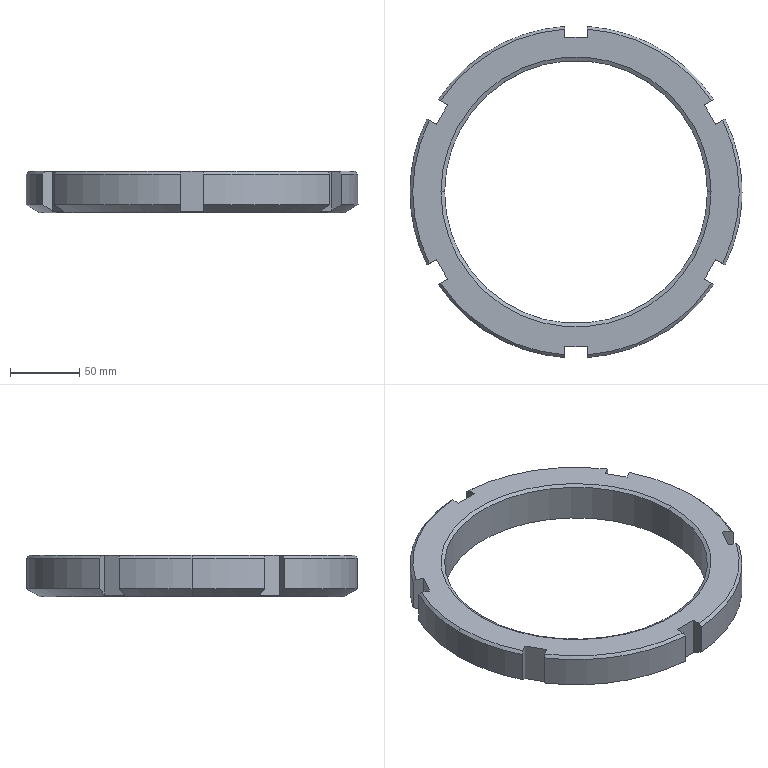Part | SolidWorks | features Chamfer 3, CirPattern 1, Cut 1, Extrusion 1 | 1 solid | 42 faces | box 240 x 239.437 x 30 mm | volume 460595 mm3 | plane 20 | cone 13 | cylinder 9 | commonest cylinder face diameters 240 x7 190 x2
STEP:
#1=CARTESIAN_POINT('',(-95.,0.,28.5));
#2=VERTEX_POINT('',#1);
#3=CARTESIAN_POINT('',(95.,0.,28.5));
#4=VERTEX_POINT('',#3);
#5=CARTESIAN_POINT('',(0.,0.,28.5));
#6=DIRECTION('',(0.,0.,1.));
#7=DIRECTION('',(1.,0.,0.));
#8=AXIS2_PLACEMENT_3D('',#5,#6,#7);
#9=CIRCLE('',#8,95.);
#10=EDGE_CURVE('',#2,#4,#9,.T.);
#11=ORIENTED_EDGE('',*,*,#10,.F.);
#12=CARTESIAN_POINT('',(-97.598,0.,30.));
#13=VERTEX_POINT('',#12);
#14=CARTESIAN_POINT('',(-95.,0.,28.5));
#15=DIRECTION('',(-0.866,0.,0.5));
#16=VECTOR('',#15,1000.);
#17=LINE('',#14,#16);
#18=EDGE_CURVE('',#2,#13,#17,.T.);
#19=ORIENTED_EDGE('',*,*,#18,.T.);
#20=CARTESIAN_POINT('',(97.598,0.,30.));
#21=VERTEX_POINT('',#20);
#22=CARTESIAN_POINT('',(0.,0.,30.));
#23=DIRECTION('',(0.,0.,-1.));
#24=DIRECTION('',(1.,0.,0.));
#25=AXIS2_PLACEMENT_3D('',#22,#23,#24);
#26=CIRCLE('',#25,97.598);
#27=EDGE_CURVE('',#21,#13,#26,.T.);
#28=ORIENTED_EDGE('',*,*,#27,.F.);
#29=CARTESIAN_POINT('',(95.,0.,28.5));
#30=DIRECTION('',(0.866,0.,0.5));
#31=VECTOR('',#30,1000.);
#32=LINE('',#29,#31);
#33=EDGE_CURVE('',#4,#21,#32,.T.);
#34=ORIENTED_EDGE('',*,*,#33,.F.);
#35=EDGE_LOOP('',(#11,#19,#28,#34));
#36=FACE_OUTER_BOUND('',#35,.T.);
#37=CARTESIAN_POINT('',(0.,0.,28.5));
#38=DIRECTION('',(0.,0.,1.));
#39=DIRECTION('',(1.,0.,0.));
#40=AXIS2_PLACEMENT_3D('',#37,#38,#39);
#41=CONICAL_SURFACE('',#40,95.,1.047);
#42=ADVANCED_FACE('',(#36),#41,.F.);
#43=CARTESIAN_POINT('',(95.,0.,1.5));
#44=VERTEX_POINT('',#43);
#45=CARTESIAN_POINT('',(-95.,0.,1.5));
#46=VERTEX_POINT('',#45);
#47=CARTESIAN_POINT('',(0.,0.,1.5));
#48=DIRECTION('',(0.,0.,-1.));
#49=DIRECTION('',(1.,0.,0.));
#50=AXIS2_PLACEMENT_3D('',#47,#48,#49);
#51=CIRCLE('',#50,95.);
#52=EDGE_CURVE('',#44,#46,#51,.T.);
#53=ORIENTED_EDGE('',*,*,#52,.F.);
#54=CARTESIAN_POINT('',(97.598,0.,0.));
#55=VERTEX_POINT('',#54);
#56=CARTESIAN_POINT('',(97.598,0.,0.));
#57=DIRECTION('',(0.866,0.,-0.5));
#58=VECTOR('',#57,1000.);
#59=LINE('',#56,#58);
#60=EDGE_CURVE('',#44,#55,#59,.T.);
#61=ORIENTED_EDGE('',*,*,#60,.T.);
#62=CARTESIAN_POINT('',(-97.598,0.,0.));
#63=VERTEX_POINT('',#62);
#64=CARTESIAN_POINT('',(0.,0.,0.));
#65=DIRECTION('',(0.,0.,1.));
#66=DIRECTION('',(1.,0.,0.));
#67=AXIS2_PLACEMENT_3D('',#64,#65,#66);
#68=CIRCLE('',#67,97.598);
#69=EDGE_CURVE('',#63,#55,#68,.T.);
#70=ORIENTED_EDGE('',*,*,#69,.F.);
#71=CARTESIAN_POINT('',(-97.598,0.,0.));
#72=DIRECTION('',(-0.866,0.,-0.5));
#73=VECTOR('',#72,1000.);
#74=LINE('',#71,#73);
#75=EDGE_CURVE('',#46,#63,#74,.T.);
#76=ORIENTED_EDGE('',*,*,#75,.F.);
#77=EDGE_LOOP('',(#53,#61,#70,#76));
#78=FACE_OUTER_BOUND('',#77,.T.);
#79=CARTESIAN_POINT('',(0.,0.,0.));
#80=DIRECTION('',(0.,0.,-1.));
#81=DIRECTION('',(-1.,0.,0.));
#82=AXIS2_PLACEMENT_3D('',#79,#80,#81);
#83=CONICAL_SURFACE('',#82,97.598,1.047);
#84=ADVANCED_FACE('',(#78),#83,.F.);
#85=CARTESIAN_POINT('',(-110.,0.,0.));
#86=VERTEX_POINT('',#85);
#87=CARTESIAN_POINT('',(110.,0.,0.));
#88=VERTEX_POINT('',#87);
#89=CARTESIAN_POINT('',(0.,0.,0.));
#90=DIRECTION('',(0.,0.,-1.));
#91=DIRECTION('',(1.,0.,0.));
#92=AXIS2_PLACEMENT_3D('',#89,#90,#91);
#93=CIRCLE('',#92,110.);
#94=EDGE_CURVE('',#86,#88,#93,.T.);
#95=ORIENTED_EDGE('',*,*,#94,.F.);
#96=CARTESIAN_POINT('',(-120.,0.,5.774));
#97=VERTEX_POINT('',#96);
#98=CARTESIAN_POINT('',(-120.,0.,5.774));
#99=DIRECTION('',(-0.866,0.,0.5));
#100=VECTOR('',#99,1000.);
#101=LINE('',#98,#100);
#102=EDGE_CURVE('',#86,#97,#101,.T.);
#103=ORIENTED_EDGE('',*,*,#102,.T.);
#104=CARTESIAN_POINT('',(-107.787,52.745,5.774));
#105=VERTEX_POINT('',#104);
#106=CARTESIAN_POINT('',(0.,0.,5.774));
#107=DIRECTION('',(0.,0.,1.));
#108=DIRECTION('',(1.,0.,0.));
#109=AXIS2_PLACEMENT_3D('',#106,#107,#108);
#110=CIRCLE('',#109,120.);
#111=EDGE_CURVE('',#105,#97,#110,.T.);
#112=ORIENTED_EDGE('',*,*,#111,.F.);
#113=CARTESIAN_POINT('',(-100.945,48.795,1.224));
#114=VERTEX_POINT('',#113);
#115=CARTESIAN_POINT('',(-100.945,48.795,1.224));
#116=CARTESIAN_POINT('',(-103.226,50.112,2.74));
#117=CARTESIAN_POINT('',(-105.506,51.428,4.257));
#118=CARTESIAN_POINT('',(-107.787,52.745,5.774));
#119=B_SPLINE_CURVE_WITH_KNOTS('',3,(#115,#116,#117,#118),.UNSPECIFIED.,.F.,.F.,(4,4),(0.000000267,0.009117),.UNSPECIFIED.);
#120=EDGE_CURVE('',#114,#105,#119,.T.);
#121=ORIENTED_EDGE('',*,*,#120,.F.);
#122=CARTESIAN_POINT('',(-92.73,63.024,1.224));
#123=VERTEX_POINT('',#122);
#124=CARTESIAN_POINT('',(-92.73,63.024,1.224));
#125=CARTESIAN_POINT('',(-95.468,58.281,0.9922));
#126=CARTESIAN_POINT('',(-98.207,53.538,0.9922));
#127=CARTESIAN_POINT('',(-100.945,48.795,1.224));
#128=B_SPLINE_CURVE_WITH_KNOTS('',3,(#124,#125,#126,#127),.UNSPECIFIED.,.F.,.F.,(4,4),(0.000000231,0.01643),.UNSPECIFIED.);
#129=EDGE_CURVE('',#123,#114,#128,.T.);
#130=ORIENTED_EDGE('',*,*,#129,.F.);
#131=CARTESIAN_POINT('',(-99.572,66.974,5.774));
#132=VERTEX_POINT('',#131);
#133=CARTESIAN_POINT('',(-99.572,66.974,5.774));
#134=CARTESIAN_POINT('',(-97.291,65.657,4.257));
#135=CARTESIAN_POINT('',(-95.011,64.34,2.74));
#136=CARTESIAN_POINT('',(-92.73,63.024,1.224));
#137=B_SPLINE_CURVE_WITH_KNOTS('',3,(#133,#134,#135,#136),.UNSPECIFIED.,.F.,.F.,(4,4),(0.000000267,0.009117),.UNSPECIFIED.);
#138=EDGE_CURVE('',#132,#123,#137,.T.);
#139=ORIENTED_EDGE('',*,*,#138,.F.);
#140=CARTESIAN_POINT('',(-8.215,119.718,5.774));
#141=VERTEX_POINT('',#140);
#142=CARTESIAN_POINT('',(0.,0.,5.774));
#143=DIRECTION('',(0.,0.,1.));
#144=DIRECTION('',(1.,0.,0.));
#145=AXIS2_PLACEMENT_3D('',#142,#143,#144);
#146=CIRCLE('',#145,120.);
#147=EDGE_CURVE('',#141,#132,#146,.T.);
#148=ORIENTED_EDGE('',*,*,#147,.F.);
#149=CARTESIAN_POINT('',(-8.215,111.818,1.224));
#150=VERTEX_POINT('',#149);
#151=CARTESIAN_POINT('',(-8.215,111.818,1.224));
#152=CARTESIAN_POINT('',(-8.215,112.097,1.384));
#153=CARTESIAN_POINT('',(-8.215,112.376,1.545));
#154=CARTESIAN_POINT('',(-8.215,112.655,1.706));
#155=CARTESIAN_POINT('',(-8.215,115.01,3.061));
#156=CARTESIAN_POINT('',(-8.215,117.364,4.417));
#157=CARTESIAN_POINT('',(-8.215,119.718,5.774));
#158=B_SPLINE_CURVE_WITH_KNOTS('',3,(#151,#152,#153,#154,#155,#156,#157),.UNSPECIFIED.,.F.,.F.,(4,3,4),(0.0177,0.01867,0.02682),.UNSPECIFIED.);
#159=EDGE_CURVE('',#150,#141,#158,.T.);
#160=ORIENTED_EDGE('',*,*,#159,.F.);
#161=CARTESIAN_POINT('',(8.215,111.818,1.224));
#162=VERTEX_POINT('',#161);
#163=CARTESIAN_POINT('',(8.215,111.818,1.224));
#164=CARTESIAN_POINT('',(5.483,111.818,1.108));
#165=CARTESIAN_POINT('',(2.747,111.818,1.05));
#166=CARTESIAN_POINT('',(-2.73,111.818,1.05));
#167=CARTESIAN_POINT('',(-5.475,111.818,1.108));
#168=CARTESIAN_POINT('',(-8.215,111.818,1.224));
#169=B_SPLINE_CURVE_WITH_KNOTS('',3,(#163,#164,#165,#166,#167,#168),.UNSPECIFIED.,.F.,.F.,(4,2,4),(0.01999,0.02819,0.0364),.UNSPECIFIED.);
#170=EDGE_CURVE('',#162,#150,#169,.T.);
#171=ORIENTED_EDGE('',*,*,#170,.F.);
#172=CARTESIAN_POINT('',(8.215,119.718,5.774));
#173=VERTEX_POINT('',#172);
#174=CARTESIAN_POINT('',(8.215,119.718,5.774));
#175=CARTESIAN_POINT('',(8.215,117.364,4.417));
#176=CARTESIAN_POINT('',(8.215,115.01,3.061));
#177=CARTESIAN_POINT('',(8.215,112.655,1.706));
#178=CARTESIAN_POINT('',(8.215,112.376,1.545));
#179=CARTESIAN_POINT('',(8.215,112.097,1.384));
#180=CARTESIAN_POINT('',(8.215,111.818,1.224));
#181=B_SPLINE_CURVE_WITH_KNOTS('',3,(#174,#175,#176,#177,#178,#179,#180),.UNSPECIFIED.,.F.,.F.,(4,3,4),(0.01052,0.01867,0.01963),.UNSPECIFIED.);
#182=EDGE_CURVE('',#173,#162,#181,.T.);
#183=ORIENTED_EDGE('',*,*,#182,.F.);
#184=CARTESIAN_POINT('',(99.572,66.974,5.774));
#185=VERTEX_POINT('',#184);
#186=CARTESIAN_POINT('',(0.,0.,5.774));
#187=DIRECTION('',(0.,0.,1.));
#188=DIRECTION('',(1.,0.,0.));
#189=AXIS2_PLACEMENT_3D('',#186,#187,#188);
#190=CIRCLE('',#189,120.);
#191=EDGE_CURVE('',#185,#173,#190,.T.);
#192=ORIENTED_EDGE('',*,*,#191,.F.);
#193=CARTESIAN_POINT('',(92.73,63.024,1.224));
#194=VERTEX_POINT('',#193);
#195=CARTESIAN_POINT('',(92.73,63.024,1.224));
#196=CARTESIAN_POINT('',(95.011,64.34,2.74));
#197=CARTESIAN_POINT('',(97.291,65.657,4.257));
#198=CARTESIAN_POINT('',(99.572,66.974,5.774));
#199=B_SPLINE_CURVE_WITH_KNOTS('',3,(#195,#196,#197,#198),.UNSPECIFIED.,.F.,.F.,(4,4),(0.000000267,0.009117),.UNSPECIFIED.);
#200=EDGE_CURVE('',#194,#185,#199,.T.);
#201=ORIENTED_EDGE('',*,*,#200,.F.);
#202=CARTESIAN_POINT('',(100.945,48.795,1.224));
#203=VERTEX_POINT('',#202);
#204=CARTESIAN_POINT('',(100.945,48.795,1.224));
#205=CARTESIAN_POINT('',(98.207,53.538,0.9922));
#206=CARTESIAN_POINT('',(95.468,58.281,0.9922));
#207=CARTESIAN_POINT('',(92.73,63.024,1.224));
#208=B_SPLINE_CURVE_WITH_KNOTS('',3,(#204,#205,#206,#207),.UNSPECIFIED.,.F.,.F.,(4,4),(0.000000231,0.01643),.UNSPECIFIED.);
#209=EDGE_CURVE('',#203,#194,#208,.T.);
#210=ORIENTED_EDGE('',*,*,#209,.F.);
#211=CARTESIAN_POINT('',(107.787,52.745,5.774));
#212=VERTEX_POINT('',#211);
#213=CARTESIAN_POINT('',(107.787,52.745,5.774));
#214=CARTESIAN_POINT('',(105.506,51.428,4.257));
#215=CARTESIAN_POINT('',(103.226,50.112,2.74));
#216=CARTESIAN_POINT('',(100.945,48.795,1.224));
#217=B_SPLINE_CURVE_WITH_KNOTS('',3,(#213,#214,#215,#216),.UNSPECIFIED.,.F.,.F.,(4,4),(0.000000267,0.009117),.UNSPECIFIED.);
#218=EDGE_CURVE('',#212,#203,#217,.T.);
#219=ORIENTED_EDGE('',*,*,#218,.F.);
#220=CARTESIAN_POINT('',(120.,0.,5.774));
#221=VERTEX_POINT('',#220);
#222=CARTESIAN_POINT('',(0.,0.,5.774));
#223=DIRECTION('',(0.,0.,1.));
#224=DIRECTION('',(1.,0.,0.));
#225=AXIS2_PLACEMENT_3D('',#222,#223,#224);
#226=CIRCLE('',#225,120.);
#227=EDGE_CURVE('',#221,#212,#226,.T.);
#228=ORIENTED_EDGE('',*,*,#227,.F.);
#229=CARTESIAN_POINT('',(120.,0.,5.774));
#230=DIRECTION('',(0.866,0.,0.5));
#231=VECTOR('',#230,1000.);
#232=LINE('',#229,#231);
#233=EDGE_CURVE('',#88,#221,#232,.T.);
#234=ORIENTED_EDGE('',*,*,#233,.F.);
#235=EDGE_LOOP('',(#95,#103,#112,#121,#130,#139,#148,#160,#171,#183,#192,#201,#210,#219,#228,#234));
#236=FACE_OUTER_BOUND('',#235,.T.);
#237=CARTESIAN_POINT('',(0.,0.,5.774));
#238=DIRECTION('',(0.,0.,1.));
#239=DIRECTION('',(1.,0.,0.));
#240=AXIS2_PLACEMENT_3D('',#237,#238,#239);
#241=CONICAL_SURFACE('',#240,120.,1.047);
#242=ADVANCED_FACE('',(#236),#241,.T.);
#243=ORIENTED_EDGE('',*,*,#10,.T.);
#244=CARTESIAN_POINT('',(95.,0.,30.));
#245=DIRECTION('',(0.,0.,-1.));
#246=VECTOR('',#245,1000.);
#247=LINE('',#244,#246);
#248=EDGE_CURVE('',#4,#44,#247,.T.);
#249=ORIENTED_EDGE('',*,*,#248,.T.);
#250=ORIENTED_EDGE('',*,*,#52,.T.);
#251=CARTESIAN_POINT('',(-95.,0.,30.));
#252=DIRECTION('',(0.,0.,-1.));
#253=VECTOR('',#252,1000.);
#254=LINE('',#251,#253);
#255=EDGE_CURVE('',#2,#46,#254,.T.);
#256=ORIENTED_EDGE('',*,*,#255,.F.);
#257=EDGE_LOOP('',(#243,#249,#250,#256));
#258=FACE_OUTER_BOUND('',#257,.T.);
#259=CARTESIAN_POINT('',(0.,0.,30.));
#260=DIRECTION('',(0.,0.,-1.));
#261=DIRECTION('',(-1.,0.,0.));
#262=AXIS2_PLACEMENT_3D('',#259,#260,#261);
#263=CYLINDRICAL_SURFACE('',#262,95.);
#264=ADVANCED_FACE('',(#258),#263,.F.);
#265=CARTESIAN_POINT('',(-118.,0.,30.));
#266=VERTEX_POINT('',#265);
#267=CARTESIAN_POINT('',(-106.051,-51.742,30.));
#268=VERTEX_POINT('',#267);
#269=CARTESIAN_POINT('',(0.,0.,30.));
#270=DIRECTION('',(0.,0.,1.));
#271=DIRECTION('',(1.,0.,0.));
#272=AXIS2_PLACEMENT_3D('',#269,#270,#271);
#273=CIRCLE('',#272,118.);
#274=EDGE_CURVE('',#266,#268,#273,.T.);
#275=ORIENTED_EDGE('',*,*,#274,.F.);
#276=CARTESIAN_POINT('',(-120.,0.,28.));
#277=VERTEX_POINT('',#276);
#278=CARTESIAN_POINT('',(-118.,0.,30.));
#279=DIRECTION('',(-0.7071,0.,-0.7071));
#280=VECTOR('',#279,1000.);
#281=LINE('',#278,#280);
#282=EDGE_CURVE('',#266,#277,#281,.T.);
#283=ORIENTED_EDGE('',*,*,#282,.T.);
#284=CARTESIAN_POINT('',(-107.787,-52.745,28.));
#285=VERTEX_POINT('',#284);
#286=CARTESIAN_POINT('',(0.,0.,28.));
#287=DIRECTION('',(0.,0.,-1.));
#288=DIRECTION('',(1.,0.,0.));
#289=AXIS2_PLACEMENT_3D('',#286,#287,#288);
#290=CIRCLE('',#289,120.);
#291=EDGE_CURVE('',#285,#277,#290,.T.);
#292=ORIENTED_EDGE('',*,*,#291,.F.);
#293=CARTESIAN_POINT('',(-106.051,-51.742,30.));
#294=CARTESIAN_POINT('',(-106.629,-52.077,29.333));
#295=CARTESIAN_POINT('',(-107.208,-52.411,28.667));
#296=CARTESIAN_POINT('',(-107.787,-52.745,28.));
#297=B_SPLINE_CURVE_WITH_KNOTS('',3,(#293,#294,#295,#296),.UNSPECIFIED.,.F.,.F.,(4,4),(0.000000283,0.002832),.UNSPECIFIED.);
#298=EDGE_CURVE('',#268,#285,#297,.T.);
#299=ORIENTED_EDGE('',*,*,#298,.F.);
#300=EDGE_LOOP('',(#275,#283,#292,#299));
#301=FACE_OUTER_BOUND('',#300,.T.);
#302=CARTESIAN_POINT('',(0.,0.,30.));
#303=DIRECTION('',(0.,0.,-1.));
#304=DIRECTION('',(-1.,0.,0.));
#305=AXIS2_PLACEMENT_3D('',#302,#303,#304);
#306=CONICAL_SURFACE('',#305,118.,0.7854);
#307=ADVANCED_FACE('',(#301),#306,.T.);
#308=ORIENTED_EDGE('',*,*,#291,.T.);
#309=CARTESIAN_POINT('',(-120.,0.,30.));
#310=DIRECTION('',(0.,0.,-1.));
#311=VECTOR('',#310,1000.);
#312=LINE('',#309,#311);
#313=EDGE_CURVE('',#277,#97,#312,.T.);
#314=ORIENTED_EDGE('',*,*,#313,.T.);
#315=CARTESIAN_POINT('',(-107.787,-52.745,5.774));
#316=VERTEX_POINT('',#315);
#317=CARTESIAN_POINT('',(0.,0.,5.774));
#318=DIRECTION('',(0.,0.,1.));
#319=DIRECTION('',(1.,0.,0.));
#320=AXIS2_PLACEMENT_3D('',#317,#318,#319);
#321=CIRCLE('',#320,120.);
#322=EDGE_CURVE('',#97,#316,#321,.T.);
#323=ORIENTED_EDGE('',*,*,#322,.T.);
#324=CARTESIAN_POINT('',(-107.787,-52.745,0.));
#325=DIRECTION('',(0.,0.,1.));
#326=VECTOR('',#325,1000.);
#327=LINE('',#324,#326);
#328=EDGE_CURVE('',#316,#285,#327,.T.);
#329=ORIENTED_EDGE('',*,*,#328,.T.);
#330=EDGE_LOOP('',(#308,#314,#323,#329));
#331=FACE_OUTER_BOUND('',#330,.T.);
#332=CARTESIAN_POINT('',(0.,0.,30.));
#333=DIRECTION('',(0.,0.,-1.));
#334=DIRECTION('',(-1.,0.,0.));
#335=AXIS2_PLACEMENT_3D('',#332,#333,#334);
#336=CYLINDRICAL_SURFACE('',#335,120.);
#337=ADVANCED_FACE('',(#331),#336,.T.);
#338=CARTESIAN_POINT('',(107.787,52.745,28.));
#339=VERTEX_POINT('',#338);
#340=CARTESIAN_POINT('',(107.787,-52.745,28.));
#341=VERTEX_POINT('',#340);
#342=CARTESIAN_POINT('',(0.,0.,28.));
#343=DIRECTION('',(0.,0.,-1.));
#344=DIRECTION('',(1.,0.,0.));
#345=AXIS2_PLACEMENT_3D('',#342,#343,#344);
#346=CIRCLE('',#345,120.);
#347=EDGE_CURVE('',#339,#341,#346,.T.);
#348=ORIENTED_EDGE('',*,*,#347,.T.);
#349=CARTESIAN_POINT('',(107.787,-52.745,5.774));
#350=VERTEX_POINT('',#349);
#351=CARTESIAN_POINT('',(107.787,-52.745,0.));
#352=DIRECTION('',(0.,0.,1.));
#353=VECTOR('',#352,1000.);
#354=LINE('',#351,#353);
#355=EDGE_CURVE('',#350,#341,#354,.T.);
#356=ORIENTED_EDGE('',*,*,#355,.F.);
#357=CARTESIAN_POINT('',(0.,0.,5.774));
#358=DIRECTION('',(0.,0.,1.));
#359=DIRECTION('',(1.,0.,0.));
#360=AXIS2_PLACEMENT_3D('',#357,#358,#359);
#361=CIRCLE('',#360,120.);
#362=EDGE_CURVE('',#350,#221,#361,.T.);
#363=ORIENTED_EDGE('',*,*,#362,.T.);
#364=ORIENTED_EDGE('',*,*,#227,.T.);
#365=CARTESIAN_POINT('',(107.787,52.745,0.));
#366=DIRECTION('',(0.,0.,1.));
#367=VECTOR('',#366,1000.);
#368=LINE('',#365,#367);
#369=EDGE_CURVE('',#212,#339,#368,.T.);
#370=ORIENTED_EDGE('',*,*,#369,.T.);
#371=EDGE_LOOP('',(#348,#356,#363,#364,#370));
#372=FACE_OUTER_BOUND('',#371,.T.);
#373=CARTESIAN_POINT('',(0.,0.,30.));
#374=DIRECTION('',(0.,0.,-1.));
#375=DIRECTION('',(-1.,0.,0.));
#376=AXIS2_PLACEMENT_3D('',#373,#374,#375);
#377=CYLINDRICAL_SURFACE('',#376,120.);
#378=ADVANCED_FACE('',(#372),#377,.T.);
#379=CARTESIAN_POINT('',(106.051,-51.742,30.));
#380=VERTEX_POINT('',#379);
#381=CARTESIAN_POINT('',(107.787,-52.745,28.));
#382=CARTESIAN_POINT('',(107.208,-52.411,28.667));
#383=CARTESIAN_POINT('',(106.629,-52.077,29.333));
#384=CARTESIAN_POINT('',(106.051,-51.742,30.));
#385=B_SPLINE_CURVE_WITH_KNOTS('',3,(#381,#382,#383,#384),.UNSPECIFIED.,.F.,.F.,(4,4),(0.000000283,0.002832),.UNSPECIFIED.);
#386=EDGE_CURVE('',#341,#380,#385,.T.);
#387=ORIENTED_EDGE('',*,*,#386,.F.);
#388=ORIENTED_EDGE('',*,*,#347,.F.);
#389=CARTESIAN_POINT('',(106.051,51.742,30.));
#390=VERTEX_POINT('',#389);
#391=CARTESIAN_POINT('',(106.051,51.742,30.));
#392=CARTESIAN_POINT('',(106.629,52.077,29.333));
#393=CARTESIAN_POINT('',(107.208,52.411,28.667));
#394=CARTESIAN_POINT('',(107.787,52.745,28.));
#395=B_SPLINE_CURVE_WITH_KNOTS('',3,(#391,#392,#393,#394),.UNSPECIFIED.,.F.,.F.,(4,4),(0.000000283,0.002832),.UNSPECIFIED.);
#396=EDGE_CURVE('',#390,#339,#395,.T.);
#397=ORIENTED_EDGE('',*,*,#396,.F.);
#398=CARTESIAN_POINT('',(0.,0.,30.));
#399=DIRECTION('',(0.,0.,1.));
#400=DIRECTION('',(1.,0.,0.));
#401=AXIS2_PLACEMENT_3D('',#398,#399,#400);
#402=CIRCLE('',#401,118.);
#403=EDGE_CURVE('',#380,#390,#402,.T.);
#404=ORIENTED_EDGE('',*,*,#403,.F.);
#405=EDGE_LOOP('',(#387,#388,#397,#404));
#406=FACE_OUTER_BOUND('',#405,.T.);
#407=CARTESIAN_POINT('',(0.,0.,30.));
#408=DIRECTION('',(0.,0.,-1.));
#409=DIRECTION('',(-1.,0.,0.));
#410=AXIS2_PLACEMENT_3D('',#407,#408,#409);
#411=CONICAL_SURFACE('',#410,118.,0.7854);
#412=ADVANCED_FACE('',(#406),#411,.T.);
#413=CARTESIAN_POINT('',(8.215,119.718,28.));
#414=VERTEX_POINT('',#413);
#415=CARTESIAN_POINT('',(99.572,66.974,28.));
#416=VERTEX_POINT('',#415);
#417=CARTESIAN_POINT('',(0.,0.,28.));
#418=DIRECTION('',(0.,0.,-1.));
#419=DIRECTION('',(1.,0.,0.));
#420=AXIS2_PLACEMENT_3D('',#417,#418,#419);
#421=CIRCLE('',#420,120.);
#422=EDGE_CURVE('',#414,#416,#421,.T.);
#423=ORIENTED_EDGE('',*,*,#422,.T.);
#424=CARTESIAN_POINT('',(99.572,66.974,0.));
#425=DIRECTION('',(0.,0.,1.));
#426=VECTOR('',#425,1000.);
#427=LINE('',#424,#426);
#428=EDGE_CURVE('',#185,#416,#427,.T.);
#429=ORIENTED_EDGE('',*,*,#428,.F.);
#430=ORIENTED_EDGE('',*,*,#191,.T.);
#431=CARTESIAN_POINT('',(8.215,119.718,0.));
#432=DIRECTION('',(0.,0.,1.));
#433=VECTOR('',#432,1000.);
#434=LINE('',#431,#433);
#435=EDGE_CURVE('',#173,#414,#434,.T.);
#436=ORIENTED_EDGE('',*,*,#435,.T.);
#437=EDGE_LOOP('',(#423,#429,#430,#436));
#438=FACE_OUTER_BOUND('',#437,.T.);
#439=CARTESIAN_POINT('',(0.,0.,30.));
#440=DIRECTION('',(0.,0.,-1.));
#441=DIRECTION('',(-1.,0.,0.));
#442=AXIS2_PLACEMENT_3D('',#439,#440,#441);
#443=CYLINDRICAL_SURFACE('',#442,120.);
#444=ADVANCED_FACE('',(#438),#443,.T.);
#445=CARTESIAN_POINT('',(97.836,65.971,30.));
#446=VERTEX_POINT('',#445);
#447=CARTESIAN_POINT('',(99.572,66.974,28.));
#448=CARTESIAN_POINT('',(98.993,66.64,28.667));
#449=CARTESIAN_POINT('',(98.414,66.305,29.333));
#450=CARTESIAN_POINT('',(97.836,65.971,30.));
#451=B_SPLINE_CURVE_WITH_KNOTS('',3,(#447,#448,#449,#450),.UNSPECIFIED.,.F.,.F.,(4,4),(0.000000283,0.002832),.UNSPECIFIED.);
#452=EDGE_CURVE('',#416,#446,#451,.T.);
#453=ORIENTED_EDGE('',*,*,#452,.F.);
#454=ORIENTED_EDGE('',*,*,#422,.F.);
#455=CARTESIAN_POINT('',(8.215,117.714,30.));
#456=VERTEX_POINT('',#455);
#457=CARTESIAN_POINT('',(8.215,117.714,30.));
#458=CARTESIAN_POINT('',(8.215,117.72,29.993));
#459=CARTESIAN_POINT('',(8.215,117.727,29.987));
#460=CARTESIAN_POINT('',(8.215,117.734,29.98));
#461=CARTESIAN_POINT('',(8.215,118.395,29.32));
#462=CARTESIAN_POINT('',(8.215,119.057,28.66));
#463=CARTESIAN_POINT('',(8.215,119.718,28.));
#464=B_SPLINE_CURVE_WITH_KNOTS('',3,(#457,#458,#459,#460,#461,#462,#463),.UNSPECIFIED.,.F.,.F.,(4,3,4),(0.01541,0.01543,0.01824),.UNSPECIFIED.);
#465=EDGE_CURVE('',#456,#414,#464,.T.);
#466=ORIENTED_EDGE('',*,*,#465,.F.);
#467=CARTESIAN_POINT('',(0.,0.,30.));
#468=DIRECTION('',(0.,0.,1.));
#469=DIRECTION('',(1.,0.,0.));
#470=AXIS2_PLACEMENT_3D('',#467,#468,#469);
#471=CIRCLE('',#470,118.);
#472=EDGE_CURVE('',#446,#456,#471,.T.);
#473=ORIENTED_EDGE('',*,*,#472,.F.);
#474=EDGE_LOOP('',(#453,#454,#466,#473));
#475=FACE_OUTER_BOUND('',#474,.T.);
#476=CARTESIAN_POINT('',(0.,0.,30.));
#477=DIRECTION('',(0.,0.,-1.));
#478=DIRECTION('',(-1.,0.,0.));
#479=AXIS2_PLACEMENT_3D('',#476,#477,#478);
#480=CONICAL_SURFACE('',#479,118.,0.7854);
#481=ADVANCED_FACE('',(#475),#480,.T.);
#482=CARTESIAN_POINT('',(-99.572,66.974,28.));
#483=VERTEX_POINT('',#482);
#484=CARTESIAN_POINT('',(-8.215,119.718,28.));
#485=VERTEX_POINT('',#484);
#486=CARTESIAN_POINT('',(0.,0.,28.));
#487=DIRECTION('',(0.,0.,-1.));
#488=DIRECTION('',(1.,0.,0.));
#489=AXIS2_PLACEMENT_3D('',#486,#487,#488);
#490=CIRCLE('',#489,120.);
#491=EDGE_CURVE('',#483,#485,#490,.T.);
#492=ORIENTED_EDGE('',*,*,#491,.T.);
#493=CARTESIAN_POINT('',(-8.215,119.718,0.));
#494=DIRECTION('',(0.,0.,1.));
#495=VECTOR('',#494,1000.);
#496=LINE('',#493,#495);
#497=EDGE_CURVE('',#141,#485,#496,.T.);
#498=ORIENTED_EDGE('',*,*,#497,.F.);
#499=ORIENTED_EDGE('',*,*,#147,.T.);
#500=CARTESIAN_POINT('',(-99.572,66.974,0.));
#501=DIRECTION('',(0.,0.,1.));
#502=VECTOR('',#501,1000.);
#503=LINE('',#500,#502);
#504=EDGE_CURVE('',#132,#483,#503,.T.);
#505=ORIENTED_EDGE('',*,*,#504,.T.);
#506=EDGE_LOOP('',(#492,#498,#499,#505));
#507=FACE_OUTER_BOUND('',#506,.T.);
#508=CARTESIAN_POINT('',(0.,0.,30.));
#509=DIRECTION('',(0.,0.,-1.));
#510=DIRECTION('',(-1.,0.,0.));
#511=AXIS2_PLACEMENT_3D('',#508,#509,#510);
#512=CYLINDRICAL_SURFACE('',#511,120.);
#513=ADVANCED_FACE('',(#507),#512,.T.);
#514=CARTESIAN_POINT('',(-8.215,117.714,30.));
#515=VERTEX_POINT('',#514);
#516=CARTESIAN_POINT('',(-8.215,119.718,28.));
#517=CARTESIAN_POINT('',(-8.215,119.057,28.66));
#518=CARTESIAN_POINT('',(-8.215,118.395,29.32));
#519=CARTESIAN_POINT('',(-8.215,117.734,29.98));
#520=CARTESIAN_POINT('',(-8.215,117.727,29.987));
#521=CARTESIAN_POINT('',(-8.215,117.72,29.993));
#522=CARTESIAN_POINT('',(-8.215,117.714,30.));
#523=B_SPLINE_CURVE_WITH_KNOTS('',3,(#516,#517,#518,#519,#520,#521,#522),.UNSPECIFIED.,.F.,.F.,(4,3,4),(0.01263,0.01543,0.01546),.UNSPECIFIED.);
#524=EDGE_CURVE('',#485,#515,#523,.T.);
#525=ORIENTED_EDGE('',*,*,#524,.F.);
#526=ORIENTED_EDGE('',*,*,#491,.F.);
#527=CARTESIAN_POINT('',(-97.836,65.971,30.));
#528=VERTEX_POINT('',#527);
#529=CARTESIAN_POINT('',(-97.836,65.971,30.));
#530=CARTESIAN_POINT('',(-98.414,66.305,29.333));
#531=CARTESIAN_POINT('',(-98.993,66.64,28.667));
#532=CARTESIAN_POINT('',(-99.572,66.974,28.));
#533=B_SPLINE_CURVE_WITH_KNOTS('',3,(#529,#530,#531,#532),.UNSPECIFIED.,.F.,.F.,(4,4),(0.000000283,0.002832),.UNSPECIFIED.);
#534=EDGE_CURVE('',#528,#483,#533,.T.);
#535=ORIENTED_EDGE('',*,*,#534,.F.);
#536=CARTESIAN_POINT('',(0.,0.,30.));
#537=DIRECTION('',(0.,0.,1.));
#538=DIRECTION('',(1.,0.,0.));
#539=AXIS2_PLACEMENT_3D('',#536,#537,#538);
#540=CIRCLE('',#539,118.);
#541=EDGE_CURVE('',#515,#528,#540,.T.);
#542=ORIENTED_EDGE('',*,*,#541,.F.);
#543=EDGE_LOOP('',(#525,#526,#535,#542));
#544=FACE_OUTER_BOUND('',#543,.T.);
#545=CARTESIAN_POINT('',(0.,0.,30.));
#546=DIRECTION('',(0.,0.,-1.));
#547=DIRECTION('',(-1.,0.,0.));
#548=AXIS2_PLACEMENT_3D('',#545,#546,#547);
#549=CONICAL_SURFACE('',#548,118.,0.7854);
#550=ADVANCED_FACE('',(#544),#549,.T.);
#551=ORIENTED_EDGE('',*,*,#313,.F.);
#552=CARTESIAN_POINT('',(-107.787,52.745,28.));
#553=VERTEX_POINT('',#552);
#554=CARTESIAN_POINT('',(0.,0.,28.));
#555=DIRECTION('',(0.,0.,-1.));
#556=DIRECTION('',(1.,0.,0.));
#557=AXIS2_PLACEMENT_3D('',#554,#555,#556);
#558=CIRCLE('',#557,120.);
#559=EDGE_CURVE('',#277,#553,#558,.T.);
#560=ORIENTED_EDGE('',*,*,#559,.T.);
#561=CARTESIAN_POINT('',(-107.787,52.745,0.));
#562=DIRECTION('',(0.,0.,1.));
#563=VECTOR('',#562,1000.);
#564=LINE('',#561,#563);
#565=EDGE_CURVE('',#105,#553,#564,.T.);
#566=ORIENTED_EDGE('',*,*,#565,.F.);
#567=ORIENTED_EDGE('',*,*,#111,.T.);
#568=EDGE_LOOP('',(#551,#560,#566,#567));
#569=FACE_OUTER_BOUND('',#568,.T.);
#570=CARTESIAN_POINT('',(0.,0.,30.));
#571=DIRECTION('',(0.,0.,-1.));
#572=DIRECTION('',(-1.,0.,0.));
#573=AXIS2_PLACEMENT_3D('',#570,#571,#572);
#574=CYLINDRICAL_SURFACE('',#573,120.);
#575=ADVANCED_FACE('',(#569),#574,.T.);
#576=ORIENTED_EDGE('',*,*,#282,.F.);
#577=CARTESIAN_POINT('',(-106.051,51.742,30.));
#578=VERTEX_POINT('',#577);
#579=CARTESIAN_POINT('',(0.,0.,30.));
#580=DIRECTION('',(0.,0.,1.));
#581=DIRECTION('',(1.,0.,0.));
#582=AXIS2_PLACEMENT_3D('',#579,#580,#581);
#583=CIRCLE('',#582,118.);
#584=EDGE_CURVE('',#578,#266,#583,.T.);
#585=ORIENTED_EDGE('',*,*,#584,.F.);
#586=CARTESIAN_POINT('',(-107.787,52.745,28.));
#587=CARTESIAN_POINT('',(-107.208,52.411,28.667));
#588=CARTESIAN_POINT('',(-106.629,52.077,29.333));
#589=CARTESIAN_POINT('',(-106.051,51.742,30.));
#590=B_SPLINE_CURVE_WITH_KNOTS('',3,(#586,#587,#588,#589),.UNSPECIFIED.,.F.,.F.,(4,4),(0.000000283,0.002832),.UNSPECIFIED.);
#591=EDGE_CURVE('',#553,#578,#590,.T.);
#592=ORIENTED_EDGE('',*,*,#591,.F.);
#593=ORIENTED_EDGE('',*,*,#559,.F.);
#594=EDGE_LOOP('',(#576,#585,#592,#593));
#595=FACE_OUTER_BOUND('',#594,.T.);
#596=CARTESIAN_POINT('',(0.,0.,30.));
#597=DIRECTION('',(0.,0.,-1.));
#598=DIRECTION('',(-1.,0.,0.));
#599=AXIS2_PLACEMENT_3D('',#596,#597,#598);
#600=CONICAL_SURFACE('',#599,118.,0.7854);
#601=ADVANCED_FACE('',(#595),#600,.T.);
#602=CARTESIAN_POINT('',(-8.215,-119.718,28.));
#603=VERTEX_POINT('',#602);
#604=CARTESIAN_POINT('',(-99.572,-66.974,28.));
#605=VERTEX_POINT('',#604);
#606=CARTESIAN_POINT('',(0.,0.,28.));
#607=DIRECTION('',(0.,0.,-1.));
#608=DIRECTION('',(1.,0.,0.));
#609=AXIS2_PLACEMENT_3D('',#606,#607,#608);
#610=CIRCLE('',#609,120.);
#611=EDGE_CURVE('',#603,#605,#610,.T.);
#612=ORIENTED_EDGE('',*,*,#611,.T.);
#613=CARTESIAN_POINT('',(-99.572,-66.974,5.774));
#614=VERTEX_POINT('',#613);
#615=CARTESIAN_POINT('',(-99.572,-66.974,0.));
#616=DIRECTION('',(0.,0.,1.));
#617=VECTOR('',#616,1000.);
#618=LINE('',#615,#617);
#619=EDGE_CURVE('',#614,#605,#618,.T.);
#620=ORIENTED_EDGE('',*,*,#619,.F.);
#621=CARTESIAN_POINT('',(-8.215,-119.718,5.774));
#622=VERTEX_POINT('',#621);
#623=CARTESIAN_POINT('',(0.,0.,5.774));
#624=DIRECTION('',(0.,0.,1.));
#625=DIRECTION('',(1.,0.,0.));
#626=AXIS2_PLACEMENT_3D('',#623,#624,#625);
#627=CIRCLE('',#626,120.);
#628=EDGE_CURVE('',#614,#622,#627,.T.);
#629=ORIENTED_EDGE('',*,*,#628,.T.);
#630=CARTESIAN_POINT('',(-8.215,-119.718,0.));
#631=DIRECTION('',(0.,0.,1.));
#632=VECTOR('',#631,1000.);
#633=LINE('',#630,#632);
#634=EDGE_CURVE('',#622,#603,#633,.T.);
#635=ORIENTED_EDGE('',*,*,#634,.T.);
#636=EDGE_LOOP('',(#612,#620,#629,#635));
#637=FACE_OUTER_BOUND('',#636,.T.);
#638=CARTESIAN_POINT('',(0.,0.,30.));
#639=DIRECTION('',(0.,0.,-1.));
#640=DIRECTION('',(-1.,0.,0.));
#641=AXIS2_PLACEMENT_3D('',#638,#639,#640);
#642=CYLINDRICAL_SURFACE('',#641,120.);
#643=ADVANCED_FACE('',(#637),#642,.T.);
#644=CARTESIAN_POINT('',(-97.836,-65.971,30.));
#645=VERTEX_POINT('',#644);
#646=CARTESIAN_POINT('',(-99.572,-66.974,28.));
#647=CARTESIAN_POINT('',(-98.993,-66.64,28.667));
#648=CARTESIAN_POINT('',(-98.414,-66.305,29.333));
#649=CARTESIAN_POINT('',(-97.836,-65.971,30.));
#650=B_SPLINE_CURVE_WITH_KNOTS('',3,(#646,#647,#648,#649),.UNSPECIFIED.,.F.,.F.,(4,4),(0.000000283,0.002832),.UNSPECIFIED.);
#651=EDGE_CURVE('',#605,#645,#650,.T.);
#652=ORIENTED_EDGE('',*,*,#651,.F.);
#653=ORIENTED_EDGE('',*,*,#611,.F.);
#654=CARTESIAN_POINT('',(-8.215,-117.714,30.));
#655=VERTEX_POINT('',#654);
#656=CARTESIAN_POINT('',(-8.215,-117.714,30.));
#657=CARTESIAN_POINT('',(-8.215,-118.05,29.664));
#658=CARTESIAN_POINT('',(-8.215,-118.387,29.328));
#659=CARTESIAN_POINT('',(-8.215,-118.724,28.993));
#660=CARTESIAN_POINT('',(-8.215,-119.055,28.662));
#661=CARTESIAN_POINT('',(-8.215,-119.387,28.331));
#662=CARTESIAN_POINT('',(-8.215,-119.718,28.));
#663=B_SPLINE_CURVE_WITH_KNOTS('',3,(#656,#657,#658,#659,#660,#661,#662),.UNSPECIFIED.,.F.,.F.,(4,3,4),(0.01401,0.01543,0.01684),.UNSPECIFIED.);
#664=EDGE_CURVE('',#655,#603,#663,.T.);
#665=ORIENTED_EDGE('',*,*,#664,.F.);
#666=CARTESIAN_POINT('',(0.,0.,30.));
#667=DIRECTION('',(0.,0.,1.));
#668=DIRECTION('',(1.,0.,0.));
#669=AXIS2_PLACEMENT_3D('',#666,#667,#668);
#670=CIRCLE('',#669,118.);
#671=EDGE_CURVE('',#645,#655,#670,.T.);
#672=ORIENTED_EDGE('',*,*,#671,.F.);
#673=EDGE_LOOP('',(#652,#653,#665,#672));
#674=FACE_OUTER_BOUND('',#673,.T.);
#675=CARTESIAN_POINT('',(0.,0.,30.));
#676=DIRECTION('',(0.,0.,-1.));
#677=DIRECTION('',(-1.,0.,0.));
#678=AXIS2_PLACEMENT_3D('',#675,#676,#677);
#679=CONICAL_SURFACE('',#678,118.,0.7854);
#680=ADVANCED_FACE('',(#674),#679,.T.);
#681=ORIENTED_EDGE('',*,*,#27,.T.);
#682=CARTESIAN_POINT('',(0.,0.,30.));
#683=DIRECTION('',(0.,0.,-1.));
#684=DIRECTION('',(1.,0.,0.));
#685=AXIS2_PLACEMENT_3D('',#682,#683,#684);
#686=CIRCLE('',#685,97.598);
#687=EDGE_CURVE('',#13,#21,#686,.T.);
#688=ORIENTED_EDGE('',*,*,#687,.T.);
#689=EDGE_LOOP('',(#681,#688));
#690=FACE_BOUND('',#689,.T.);
#691=CARTESIAN_POINT('',(100.945,-48.795,30.));
#692=VERTEX_POINT('',#691);
#693=CARTESIAN_POINT('',(100.945,-48.795,30.));
#694=DIRECTION('',(-0.866,0.5,0.));
#695=VECTOR('',#694,1000.);
#696=LINE('',#693,#695);
#697=EDGE_CURVE('',#380,#692,#696,.T.);
#698=ORIENTED_EDGE('',*,*,#697,.F.);
#699=ORIENTED_EDGE('',*,*,#403,.T.);
#700=CARTESIAN_POINT('',(100.945,48.795,30.));
#701=VERTEX_POINT('',#700);
#702=CARTESIAN_POINT('',(100.945,48.795,30.));
#703=DIRECTION('',(0.866,0.5,0.));
#704=VECTOR('',#703,1000.);
#705=LINE('',#702,#704);
#706=EDGE_CURVE('',#701,#390,#705,.T.);
#707=ORIENTED_EDGE('',*,*,#706,.F.);
#708=CARTESIAN_POINT('',(92.73,63.024,30.));
#709=VERTEX_POINT('',#708);
#710=CARTESIAN_POINT('',(100.945,48.795,30.));
#711=DIRECTION('',(0.5,-0.866,0.));
#712=VECTOR('',#711,1000.);
#713=LINE('',#710,#712);
#714=EDGE_CURVE('',#709,#701,#713,.T.);
#715=ORIENTED_EDGE('',*,*,#714,.F.);
#716=CARTESIAN_POINT('',(92.73,63.024,30.));
#717=DIRECTION('',(-0.866,-0.5,0.));
#718=VECTOR('',#717,1000.);
#719=LINE('',#716,#718);
#720=EDGE_CURVE('',#446,#709,#719,.T.);
#721=ORIENTED_EDGE('',*,*,#720,.F.);
#722=ORIENTED_EDGE('',*,*,#472,.T.);
#723=CARTESIAN_POINT('',(8.215,111.818,30.));
#724=VERTEX_POINT('',#723);
#725=CARTESIAN_POINT('',(8.215,111.818,30.));
#726=DIRECTION('',(0.,1.,0.));
#727=VECTOR('',#726,1000.);
#728=LINE('',#725,#727);
#729=EDGE_CURVE('',#724,#456,#728,.T.);
#730=ORIENTED_EDGE('',*,*,#729,.F.);
#731=CARTESIAN_POINT('',(-8.215,111.818,30.));
#732=VERTEX_POINT('',#731);
#733=CARTESIAN_POINT('',(8.215,111.818,30.));
#734=DIRECTION('',(1.,0.,0.));
#735=VECTOR('',#734,1000.);
#736=LINE('',#733,#735);
#737=EDGE_CURVE('',#732,#724,#736,.T.);
#738=ORIENTED_EDGE('',*,*,#737,.F.);
#739=CARTESIAN_POINT('',(-8.215,111.818,30.));
#740=DIRECTION('',(0.,-1.,0.));
#741=VECTOR('',#740,1000.);
#742=LINE('',#739,#741);
#743=EDGE_CURVE('',#515,#732,#742,.T.);
#744=ORIENTED_EDGE('',*,*,#743,.F.);
#745=ORIENTED_EDGE('',*,*,#541,.T.);
#746=CARTESIAN_POINT('',(-92.73,63.024,30.));
#747=VERTEX_POINT('',#746);
#748=CARTESIAN_POINT('',(-92.73,63.024,30.));
#749=DIRECTION('',(-0.866,0.5,0.));
#750=VECTOR('',#749,1000.);
#751=LINE('',#748,#750);
#752=EDGE_CURVE('',#747,#528,#751,.T.);
#753=ORIENTED_EDGE('',*,*,#752,.F.);
#754=CARTESIAN_POINT('',(-100.945,48.795,30.));
#755=VERTEX_POINT('',#754);
#756=CARTESIAN_POINT('',(-92.73,63.024,30.));
#757=DIRECTION('',(0.5,0.866,0.));
#758=VECTOR('',#757,1000.);
#759=LINE('',#756,#758);
#760=EDGE_CURVE('',#755,#747,#759,.T.);
#761=ORIENTED_EDGE('',*,*,#760,.F.);
#762=CARTESIAN_POINT('',(-100.945,48.795,30.));
#763=DIRECTION('',(0.866,-0.5,0.));
#764=VECTOR('',#763,1000.);
#765=LINE('',#762,#764);
#766=EDGE_CURVE('',#578,#755,#765,.T.);
#767=ORIENTED_EDGE('',*,*,#766,.F.);
#768=ORIENTED_EDGE('',*,*,#584,.T.);
#769=ORIENTED_EDGE('',*,*,#274,.T.);
#770=CARTESIAN_POINT('',(-100.945,-48.795,30.));
#771=VERTEX_POINT('',#770);
#772=CARTESIAN_POINT('',(-100.945,-48.795,30.));
#773=DIRECTION('',(-0.866,-0.5,0.));
#774=VECTOR('',#773,1000.);
#775=LINE('',#772,#774);
#776=EDGE_CURVE('',#771,#268,#775,.T.);
#777=ORIENTED_EDGE('',*,*,#776,.F.);
#778=CARTESIAN_POINT('',(-92.73,-63.024,30.));
#779=VERTEX_POINT('',#778);
#780=CARTESIAN_POINT('',(-100.945,-48.795,30.));
#781=DIRECTION('',(-0.5,0.866,0.));
#782=VECTOR('',#781,1000.);
#783=LINE('',#780,#782);
#784=EDGE_CURVE('',#779,#771,#783,.T.);
#785=ORIENTED_EDGE('',*,*,#784,.F.);
#786=CARTESIAN_POINT('',(-92.73,-63.024,30.));
#787=DIRECTION('',(0.866,0.5,0.));
#788=VECTOR('',#787,1000.);
#789=LINE('',#786,#788);
#790=EDGE_CURVE('',#645,#779,#789,.T.);
#791=ORIENTED_EDGE('',*,*,#790,.F.);
#792=ORIENTED_EDGE('',*,*,#671,.T.);
#793=CARTESIAN_POINT('',(-8.215,-111.818,30.));
#794=VERTEX_POINT('',#793);
#795=CARTESIAN_POINT('',(-8.215,-111.818,30.));
#796=DIRECTION('',(0.,-1.,0.));
#797=VECTOR('',#796,1000.);
#798=LINE('',#795,#797);
#799=EDGE_CURVE('',#794,#655,#798,.T.);
#800=ORIENTED_EDGE('',*,*,#799,.F.);
#801=CARTESIAN_POINT('',(8.215,-111.818,30.));
#802=VERTEX_POINT('',#801);
#803=CARTESIAN_POINT('',(-8.215,-111.818,30.));
#804=DIRECTION('',(-1.,0.,0.));
#805=VECTOR('',#804,1000.);
#806=LINE('',#803,#805);
#807=EDGE_CURVE('',#802,#794,#806,.T.);
#808=ORIENTED_EDGE('',*,*,#807,.F.);
#809=CARTESIAN_POINT('',(8.215,-117.714,30.));
#810=VERTEX_POINT('',#809);
#811=CARTESIAN_POINT('',(8.215,-111.818,30.));
#812=DIRECTION('',(0.,1.,0.));
#813=VECTOR('',#812,1000.);
#814=LINE('',#811,#813);
#815=EDGE_CURVE('',#810,#802,#814,.T.);
#816=ORIENTED_EDGE('',*,*,#815,.F.);
#817=CARTESIAN_POINT('',(97.836,-65.971,30.));
#818=VERTEX_POINT('',#817);
#819=CARTESIAN_POINT('',(0.,0.,30.));
#820=DIRECTION('',(0.,0.,1.));
#821=DIRECTION('',(1.,0.,0.));
#822=AXIS2_PLACEMENT_3D('',#819,#820,#821);
#823=CIRCLE('',#822,118.);
#824=EDGE_CURVE('',#810,#818,#823,.T.);
#825=ORIENTED_EDGE('',*,*,#824,.T.);
#826=CARTESIAN_POINT('',(92.73,-63.024,30.));
#827=VERTEX_POINT('',#826);
#828=CARTESIAN_POINT('',(92.73,-63.024,30.));
#829=DIRECTION('',(0.866,-0.5,0.));
#830=VECTOR('',#829,1000.);
#831=LINE('',#828,#830);
#832=EDGE_CURVE('',#827,#818,#831,.T.);
#833=ORIENTED_EDGE('',*,*,#832,.F.);
#834=CARTESIAN_POINT('',(92.73,-63.024,30.));
#835=DIRECTION('',(-0.5,-0.866,0.));
#836=VECTOR('',#835,1000.);
#837=LINE('',#834,#836);
#838=EDGE_CURVE('',#692,#827,#837,.T.);
#839=ORIENTED_EDGE('',*,*,#838,.F.);
#840=EDGE_LOOP('',(#698,#699,#707,#715,#721,#722,#730,#738,#744,#745,#753,#761,#767,#768,#769,#777,#785,#791,#792,#800,#808,#816,#825,#833,#839));
#841=FACE_OUTER_BOUND('',#840,.T.);
#842=CARTESIAN_POINT('',(0.,0.,30.));
#843=DIRECTION('',(0.,0.,1.));
#844=DIRECTION('',(1.,0.,0.));
#845=AXIS2_PLACEMENT_3D('',#842,#843,#844);
#846=PLANE('',#845);
#847=ADVANCED_FACE('',(#690,#841),#846,.T.);
#848=ORIENTED_EDGE('',*,*,#69,.T.);
#849=CARTESIAN_POINT('',(0.,0.,0.));
#850=DIRECTION('',(0.,0.,1.));
#851=DIRECTION('',(1.,0.,0.));
#852=AXIS2_PLACEMENT_3D('',#849,#850,#851);
#853=CIRCLE('',#852,97.598);
#854=EDGE_CURVE('',#55,#63,#853,.T.);
#855=ORIENTED_EDGE('',*,*,#854,.T.);
#856=EDGE_LOOP('',(#848,#855));
#857=FACE_BOUND('',#856,.T.);
#858=CARTESIAN_POINT('',(0.,0.,0.));
#859=DIRECTION('',(0.,0.,-1.));
#860=DIRECTION('',(1.,0.,0.));
#861=AXIS2_PLACEMENT_3D('',#858,#859,#860);
#862=CIRCLE('',#861,110.);
#863=EDGE_CURVE('',#88,#86,#862,.T.);
#864=ORIENTED_EDGE('',*,*,#863,.T.);
#865=ORIENTED_EDGE('',*,*,#94,.T.);
#866=EDGE_LOOP('',(#864,#865));
#867=FACE_OUTER_BOUND('',#866,.T.);
#868=CARTESIAN_POINT('',(0.,0.,0.));
#869=DIRECTION('',(0.,0.,1.));
#870=DIRECTION('',(1.,0.,0.));
#871=AXIS2_PLACEMENT_3D('',#868,#869,#870);
#872=PLANE('',#871);
#873=ADVANCED_FACE('',(#857,#867),#872,.F.);
#874=CARTESIAN_POINT('',(8.215,-119.718,5.774));
#875=VERTEX_POINT('',#874);
#876=CARTESIAN_POINT('',(99.572,-66.974,5.774));
#877=VERTEX_POINT('',#876);
#878=CARTESIAN_POINT('',(0.,0.,5.774));
#879=DIRECTION('',(0.,0.,1.));
#880=DIRECTION('',(1.,0.,0.));
#881=AXIS2_PLACEMENT_3D('',#878,#879,#880);
#882=CIRCLE('',#881,120.);
#883=EDGE_CURVE('',#875,#877,#882,.T.);
#884=ORIENTED_EDGE('',*,*,#883,.T.);
#885=CARTESIAN_POINT('',(99.572,-66.974,28.));
#886=VERTEX_POINT('',#885);
#887=CARTESIAN_POINT('',(99.572,-66.974,0.));
#888=DIRECTION('',(0.,0.,1.));
#889=VECTOR('',#888,1000.);
#890=LINE('',#887,#889);
#891=EDGE_CURVE('',#877,#886,#890,.T.);
#892=ORIENTED_EDGE('',*,*,#891,.T.);
#893=CARTESIAN_POINT('',(8.215,-119.718,28.));
#894=VERTEX_POINT('',#893);
#895=CARTESIAN_POINT('',(0.,0.,28.));
#896=DIRECTION('',(0.,0.,-1.));
#897=DIRECTION('',(1.,0.,0.));
#898=AXIS2_PLACEMENT_3D('',#895,#896,#897);
#899=CIRCLE('',#898,120.);
#900=EDGE_CURVE('',#886,#894,#899,.T.);
#901=ORIENTED_EDGE('',*,*,#900,.T.);
#902=CARTESIAN_POINT('',(8.215,-119.718,0.));
#903=DIRECTION('',(0.,0.,1.));
#904=VECTOR('',#903,1000.);
#905=LINE('',#902,#904);
#906=EDGE_CURVE('',#875,#894,#905,.T.);
#907=ORIENTED_EDGE('',*,*,#906,.F.);
#908=EDGE_LOOP('',(#884,#892,#901,#907));
#909=FACE_OUTER_BOUND('',#908,.T.);
#910=CARTESIAN_POINT('',(0.,0.,30.));
#911=DIRECTION('',(0.,0.,-1.));
#912=DIRECTION('',(-1.,0.,0.));
#913=AXIS2_PLACEMENT_3D('',#910,#911,#912);
#914=CYLINDRICAL_SURFACE('',#913,120.);
#915=ADVANCED_FACE('',(#909),#914,.T.);
#916=ORIENTED_EDGE('',*,*,#248,.F.);
#917=CARTESIAN_POINT('',(0.,0.,28.5));
#918=DIRECTION('',(0.,0.,1.));
#919=DIRECTION('',(1.,0.,0.));
#920=AXIS2_PLACEMENT_3D('',#917,#918,#919);
#921=CIRCLE('',#920,95.);
#922=EDGE_CURVE('',#4,#2,#921,.T.);
#923=ORIENTED_EDGE('',*,*,#922,.T.);
#924=ORIENTED_EDGE('',*,*,#255,.T.);
#925=CARTESIAN_POINT('',(0.,0.,1.5));
#926=DIRECTION('',(0.,0.,-1.));
#927=DIRECTION('',(1.,0.,0.));
#928=AXIS2_PLACEMENT_3D('',#925,#926,#927);
#929=CIRCLE('',#928,95.);
#930=EDGE_CURVE('',#46,#44,#929,.T.);
#931=ORIENTED_EDGE('',*,*,#930,.T.);
#932=EDGE_LOOP('',(#916,#923,#924,#931));
#933=FACE_OUTER_BOUND('',#932,.T.);
#934=CARTESIAN_POINT('',(0.,0.,30.));
#935=DIRECTION('',(0.,0.,-1.));
#936=DIRECTION('',(-1.,0.,0.));
#937=AXIS2_PLACEMENT_3D('',#934,#935,#936);
#938=CYLINDRICAL_SURFACE('',#937,95.);
#939=ADVANCED_FACE('',(#933),#938,.F.);
#940=CARTESIAN_POINT('',(97.836,-65.971,30.));
#941=CARTESIAN_POINT('',(98.414,-66.305,29.333));
#942=CARTESIAN_POINT('',(98.993,-66.64,28.667));
#943=CARTESIAN_POINT('',(99.572,-66.974,28.));
#944=B_SPLINE_CURVE_WITH_KNOTS('',3,(#940,#941,#942,#943),.UNSPECIFIED.,.F.,.F.,(4,4),(0.000000283,0.002832),.UNSPECIFIED.);
#945=EDGE_CURVE('',#818,#886,#944,.T.);
#946=ORIENTED_EDGE('',*,*,#945,.F.);
#947=ORIENTED_EDGE('',*,*,#824,.F.);
#948=CARTESIAN_POINT('',(8.215,-119.718,28.));
#949=CARTESIAN_POINT('',(8.215,-119.387,28.331));
#950=CARTESIAN_POINT('',(8.215,-119.055,28.662));
#951=CARTESIAN_POINT('',(8.215,-118.724,28.993));
#952=CARTESIAN_POINT('',(8.215,-118.387,29.328));
#953=CARTESIAN_POINT('',(8.215,-118.05,29.664));
#954=CARTESIAN_POINT('',(8.215,-117.714,30.));
#955=B_SPLINE_CURVE_WITH_KNOTS('',3,(#948,#949,#950,#951,#952,#953,#954),.UNSPECIFIED.,.F.,.F.,(4,3,4),(0.01403,0.01543,0.01686),.UNSPECIFIED.);
#956=EDGE_CURVE('',#894,#810,#955,.T.);
#957=ORIENTED_EDGE('',*,*,#956,.F.);
#958=ORIENTED_EDGE('',*,*,#900,.F.);
#959=EDGE_LOOP('',(#946,#947,#957,#958));
#960=FACE_OUTER_BOUND('',#959,.T.);
#961=CARTESIAN_POINT('',(0.,0.,30.));
#962=DIRECTION('',(0.,0.,-1.));
#963=DIRECTION('',(-1.,0.,0.));
#964=AXIS2_PLACEMENT_3D('',#961,#962,#963);
#965=CONICAL_SURFACE('',#964,118.,0.7854);
#966=ADVANCED_FACE('',(#960),#965,.T.);
#967=ORIENTED_EDGE('',*,*,#102,.F.);
#968=ORIENTED_EDGE('',*,*,#863,.F.);
#969=ORIENTED_EDGE('',*,*,#233,.T.);
#970=ORIENTED_EDGE('',*,*,#362,.F.);
#971=CARTESIAN_POINT('',(100.945,-48.795,1.224));
#972=VERTEX_POINT('',#971);
#973=CARTESIAN_POINT('',(100.945,-48.795,1.224));
#974=CARTESIAN_POINT('',(103.226,-50.112,2.74));
#975=CARTESIAN_POINT('',(105.506,-51.428,4.257));
#976=CARTESIAN_POINT('',(107.787,-52.745,5.774));
#977=B_SPLINE_CURVE_WITH_KNOTS('',3,(#973,#974,#975,#976),.UNSPECIFIED.,.F.,.F.,(4,4),(0.000000267,0.009117),.UNSPECIFIED.);
#978=EDGE_CURVE('',#972,#350,#977,.T.);
#979=ORIENTED_EDGE('',*,*,#978,.F.);
#980=CARTESIAN_POINT('',(92.73,-63.024,1.224));
#981=VERTEX_POINT('',#980);
#982=CARTESIAN_POINT('',(92.73,-63.024,1.224));
#983=CARTESIAN_POINT('',(95.468,-58.281,0.9922));
#984=CARTESIAN_POINT('',(98.207,-53.538,0.9922));
#985=CARTESIAN_POINT('',(100.945,-48.795,1.224));
#986=B_SPLINE_CURVE_WITH_KNOTS('',3,(#982,#983,#984,#985),.UNSPECIFIED.,.F.,.F.,(4,4),(0.000000231,0.01643),.UNSPECIFIED.);
#987=EDGE_CURVE('',#981,#972,#986,.T.);
#988=ORIENTED_EDGE('',*,*,#987,.F.);
#989=CARTESIAN_POINT('',(99.572,-66.974,5.774));
#990=CARTESIAN_POINT('',(97.291,-65.657,4.257));
#991=CARTESIAN_POINT('',(95.011,-64.34,2.74));
#992=CARTESIAN_POINT('',(92.73,-63.024,1.224));
#993=B_SPLINE_CURVE_WITH_KNOTS('',3,(#989,#990,#991,#992),.UNSPECIFIED.,.F.,.F.,(4,4),(0.000000267,0.009117),.UNSPECIFIED.);
#994=EDGE_CURVE('',#877,#981,#993,.T.);
#995=ORIENTED_EDGE('',*,*,#994,.F.);
#996=ORIENTED_EDGE('',*,*,#883,.F.);
#997=CARTESIAN_POINT('',(8.215,-111.818,1.224));
#998=VERTEX_POINT('',#997);
#999=CARTESIAN_POINT('',(8.215,-111.818,1.224));
#1000=CARTESIAN_POINT('',(8.215,-113.997,2.478));
#1001=CARTESIAN_POINT('',(8.215,-116.175,3.732));
#1002=CARTESIAN_POINT('',(8.215,-118.353,4.987));
#1003=CARTESIAN_POINT('',(8.215,-118.808,5.249));
#1004=CARTESIAN_POINT('',(8.215,-119.263,5.511));
#1005=CARTESIAN_POINT('',(8.215,-119.718,5.774));
#1006=B_SPLINE_CURVE_WITH_KNOTS('',3,(#999,#1000,#1001,#1002,#1003,#1004,#1005),.UNSPECIFIED.,.F.,.F.,(4,3,4),(0.01113,0.01867,0.02024),.UNSPECIFIED.);
#1007=EDGE_CURVE('',#998,#875,#1006,.T.);
#1008=ORIENTED_EDGE('',*,*,#1007,.F.);
#1009=CARTESIAN_POINT('',(-8.215,-111.818,1.224));
#1010=VERTEX_POINT('',#1009);
#1011=CARTESIAN_POINT('',(-8.215,-111.818,1.224));
#1012=CARTESIAN_POINT('',(-5.475,-111.818,1.108));
#1013=CARTESIAN_POINT('',(-2.73,-111.818,1.05));
#1014=CARTESIAN_POINT('',(2.747,-111.818,1.05));
#1015=CARTESIAN_POINT('',(5.483,-111.818,1.108));
#1016=CARTESIAN_POINT('',(8.215,-111.818,1.224));
#1017=B_SPLINE_CURVE_WITH_KNOTS('',3,(#1011,#1012,#1013,#1014,#1015,#1016),.UNSPECIFIED.,.F.,.F.,(4,2,4),(0.0324,0.04061,0.04881),.UNSPECIFIED.);
#1018=EDGE_CURVE('',#1010,#998,#1017,.T.);
#1019=ORIENTED_EDGE('',*,*,#1018,.F.);
#1020=CARTESIAN_POINT('',(-8.215,-119.718,5.774));
#1021=CARTESIAN_POINT('',(-8.215,-119.263,5.511));
#1022=CARTESIAN_POINT('',(-8.215,-118.808,5.249));
#1023=CARTESIAN_POINT('',(-8.215,-118.353,4.987));
#1024=CARTESIAN_POINT('',(-8.215,-116.175,3.732));
#1025=CARTESIAN_POINT('',(-8.215,-113.997,2.478));
#1026=CARTESIAN_POINT('',(-8.215,-111.818,1.224));
#1027=B_SPLINE_CURVE_WITH_KNOTS('',3,(#1020,#1021,#1022,#1023,#1024,#1025,#1026),.UNSPECIFIED.,.F.,.F.,(4,3,4),(0.01709,0.01867,0.02621),.UNSPECIFIED.);
#1028=EDGE_CURVE('',#622,#1010,#1027,.T.);
#1029=ORIENTED_EDGE('',*,*,#1028,.F.);
#1030=ORIENTED_EDGE('',*,*,#628,.F.);
#1031=CARTESIAN_POINT('',(-92.73,-63.024,1.224));
#1032=VERTEX_POINT('',#1031);
#1033=CARTESIAN_POINT('',(-92.73,-63.024,1.224));
#1034=CARTESIAN_POINT('',(-95.011,-64.34,2.74));
#1035=CARTESIAN_POINT('',(-97.291,-65.657,4.257));
#1036=CARTESIAN_POINT('',(-99.572,-66.974,5.774));
#1037=B_SPLINE_CURVE_WITH_KNOTS('',3,(#1033,#1034,#1035,#1036),.UNSPECIFIED.,.F.,.F.,(4,4),(0.000000267,0.009117),.UNSPECIFIED.);
#1038=EDGE_CURVE('',#1032,#614,#1037,.T.);
#1039=ORIENTED_EDGE('',*,*,#1038,.F.);
#1040=CARTESIAN_POINT('',(-100.945,-48.795,1.224));
#1041=VERTEX_POINT('',#1040);
#1042=CARTESIAN_POINT('',(-100.945,-48.795,1.224));
#1043=CARTESIAN_POINT('',(-98.207,-53.538,0.9922));
#1044=CARTESIAN_POINT('',(-95.468,-58.281,0.9922));
#1045=CARTESIAN_POINT('',(-92.73,-63.024,1.224));
#1046=B_SPLINE_CURVE_WITH_KNOTS('',3,(#1042,#1043,#1044,#1045),.UNSPECIFIED.,.F.,.F.,(4,4),(0.000000231,0.01643),.UNSPECIFIED.);
#1047=EDGE_CURVE('',#1041,#1032,#1046,.T.);
#1048=ORIENTED_EDGE('',*,*,#1047,.F.);
#1049=CARTESIAN_POINT('',(-107.787,-52.745,5.774));
#1050=CARTESIAN_POINT('',(-105.506,-51.428,4.257));
#1051=CARTESIAN_POINT('',(-103.226,-50.112,2.74));
#1052=CARTESIAN_POINT('',(-100.945,-48.795,1.224));
#1053=B_SPLINE_CURVE_WITH_KNOTS('',3,(#1049,#1050,#1051,#1052),.UNSPECIFIED.,.F.,.F.,(4,4),(0.000000267,0.009117),.UNSPECIFIED.);
#1054=EDGE_CURVE('',#316,#1041,#1053,.T.);
#1055=ORIENTED_EDGE('',*,*,#1054,.F.);
#1056=ORIENTED_EDGE('',*,*,#322,.F.);
#1057=EDGE_LOOP('',(#967,#968,#969,#970,#979,#988,#995,#996,#1008,#1019,#1029,#1030,#1039,#1048,#1055,#1056));
#1058=FACE_OUTER_BOUND('',#1057,.T.);
#1059=CARTESIAN_POINT('',(0.,0.,5.774));
#1060=DIRECTION('',(0.,0.,1.));
#1061=DIRECTION('',(1.,0.,0.));
#1062=AXIS2_PLACEMENT_3D('',#1059,#1060,#1061);
#1063=CONICAL_SURFACE('',#1062,120.,1.047);
#1064=ADVANCED_FACE('',(#1058),#1063,.T.);
#1065=ORIENTED_EDGE('',*,*,#1018,.T.);
#1066=CARTESIAN_POINT('',(8.215,-111.818,0.));
#1067=DIRECTION('',(0.,0.,1.));
#1068=VECTOR('',#1067,1000.);
#1069=LINE('',#1066,#1068);
#1070=EDGE_CURVE('',#998,#802,#1069,.T.);
#1071=ORIENTED_EDGE('',*,*,#1070,.T.);
#1072=ORIENTED_EDGE('',*,*,#807,.T.);
#1073=CARTESIAN_POINT('',(-8.215,-111.818,0.));
#1074=DIRECTION('',(0.,0.,1.));
#1075=VECTOR('',#1074,1000.);
#1076=LINE('',#1073,#1075);
#1077=EDGE_CURVE('',#1010,#794,#1076,.T.);
#1078=ORIENTED_EDGE('',*,*,#1077,.F.);
#1079=EDGE_LOOP('',(#1065,#1071,#1072,#1078));
#1080=FACE_OUTER_BOUND('',#1079,.T.);
#1081=CARTESIAN_POINT('',(-8.215,-111.818,0.));
#1082=DIRECTION('',(0.,1.,0.));
#1083=DIRECTION('',(0.,0.,1.));
#1084=AXIS2_PLACEMENT_3D('',#1081,#1082,#1083);
#1085=PLANE('',#1084);
#1086=ADVANCED_FACE('',(#1080),#1085,.F.);
#1087=ORIENTED_EDGE('',*,*,#956,.T.);
#1088=ORIENTED_EDGE('',*,*,#815,.T.);
#1089=ORIENTED_EDGE('',*,*,#1070,.F.);
#1090=ORIENTED_EDGE('',*,*,#1007,.T.);
#1091=ORIENTED_EDGE('',*,*,#906,.T.);
#1092=EDGE_LOOP('',(#1087,#1088,#1089,#1090,#1091));
#1093=FACE_OUTER_BOUND('',#1092,.T.);
#1094=CARTESIAN_POINT('',(8.215,-111.818,0.));
#1095=DIRECTION('',(1.,0.,0.));
#1096=DIRECTION('',(0.,1.,0.));
#1097=AXIS2_PLACEMENT_3D('',#1094,#1095,#1096);
#1098=PLANE('',#1097);
#1099=ADVANCED_FACE('',(#1093),#1098,.F.);
#1100=ORIENTED_EDGE('',*,*,#664,.T.);
#1101=ORIENTED_EDGE('',*,*,#634,.F.);
#1102=ORIENTED_EDGE('',*,*,#1028,.T.);
#1103=ORIENTED_EDGE('',*,*,#1077,.T.);
#1104=ORIENTED_EDGE('',*,*,#799,.T.);
#1105=EDGE_LOOP('',(#1100,#1101,#1102,#1103,#1104));
#1106=FACE_OUTER_BOUND('',#1105,.T.);
#1107=CARTESIAN_POINT('',(-8.215,-111.818,0.));
#1108=DIRECTION('',(-1.,0.,0.));
#1109=DIRECTION('',(0.,-1.,0.));
#1110=AXIS2_PLACEMENT_3D('',#1107,#1108,#1109);
#1111=PLANE('',#1110);
#1112=ADVANCED_FACE('',(#1106),#1111,.F.);
#1113=ORIENTED_EDGE('',*,*,#1047,.T.);
#1114=CARTESIAN_POINT('',(-92.73,-63.024,0.));
#1115=DIRECTION('',(0.,0.,1.));
#1116=VECTOR('',#1115,1000.);
#1117=LINE('',#1114,#1116);
#1118=EDGE_CURVE('',#1032,#779,#1117,.T.);
#1119=ORIENTED_EDGE('',*,*,#1118,.T.);
#1120=ORIENTED_EDGE('',*,*,#784,.T.);
#1121=CARTESIAN_POINT('',(-100.945,-48.795,0.));
#1122=DIRECTION('',(0.,0.,1.));
#1123=VECTOR('',#1122,1000.);
#1124=LINE('',#1121,#1123);
#1125=EDGE_CURVE('',#1041,#771,#1124,.T.);
#1126=ORIENTED_EDGE('',*,*,#1125,.F.);
#1127=EDGE_LOOP('',(#1113,#1119,#1120,#1126));
#1128=FACE_OUTER_BOUND('',#1127,.T.);
#1129=CARTESIAN_POINT('',(-100.945,-48.795,0.));
#1130=DIRECTION('',(0.866,0.5,0.));
#1131=DIRECTION('',(-0.5,0.866,0.));
#1132=AXIS2_PLACEMENT_3D('',#1129,#1130,#1131);
#1133=PLANE('',#1132);
#1134=ADVANCED_FACE('',(#1128),#1133,.F.);
#1135=ORIENTED_EDGE('',*,*,#651,.T.);
#1136=ORIENTED_EDGE('',*,*,#790,.T.);
#1137=ORIENTED_EDGE('',*,*,#1118,.F.);
#1138=ORIENTED_EDGE('',*,*,#1038,.T.);
#1139=ORIENTED_EDGE('',*,*,#619,.T.);
#1140=EDGE_LOOP('',(#1135,#1136,#1137,#1138,#1139));
#1141=FACE_OUTER_BOUND('',#1140,.T.);
#1142=CARTESIAN_POINT('',(-92.73,-63.024,0.));
#1143=DIRECTION('',(0.5,-0.866,0.));
#1144=DIRECTION('',(0.866,0.5,0.));
#1145=AXIS2_PLACEMENT_3D('',#1142,#1143,#1144);
#1146=PLANE('',#1145);
#1147=ADVANCED_FACE('',(#1141),#1146,.F.);
#1148=ORIENTED_EDGE('',*,*,#298,.T.);
#1149=ORIENTED_EDGE('',*,*,#328,.F.);
#1150=ORIENTED_EDGE('',*,*,#1054,.T.);
#1151=ORIENTED_EDGE('',*,*,#1125,.T.);
#1152=ORIENTED_EDGE('',*,*,#776,.T.);
#1153=EDGE_LOOP('',(#1148,#1149,#1150,#1151,#1152));
#1154=FACE_OUTER_BOUND('',#1153,.T.);
#1155=CARTESIAN_POINT('',(-100.945,-48.795,0.));
#1156=DIRECTION('',(-0.5,0.866,0.));
#1157=DIRECTION('',(-0.866,-0.5,0.));
#1158=AXIS2_PLACEMENT_3D('',#1155,#1156,#1157);
#1159=PLANE('',#1158);
#1160=ADVANCED_FACE('',(#1154),#1159,.F.);
#1161=ORIENTED_EDGE('',*,*,#129,.T.);
#1162=CARTESIAN_POINT('',(-100.945,48.795,0.));
#1163=DIRECTION('',(0.,0.,1.));
#1164=VECTOR('',#1163,1000.);
#1165=LINE('',#1162,#1164);
#1166=EDGE_CURVE('',#114,#755,#1165,.T.);
#1167=ORIENTED_EDGE('',*,*,#1166,.T.);
#1168=ORIENTED_EDGE('',*,*,#760,.T.);
#1169=CARTESIAN_POINT('',(-92.73,63.024,0.));
#1170=DIRECTION('',(0.,0.,1.));
#1171=VECTOR('',#1170,1000.);
#1172=LINE('',#1169,#1171);
#1173=EDGE_CURVE('',#123,#747,#1172,.T.);
#1174=ORIENTED_EDGE('',*,*,#1173,.F.);
#1175=EDGE_LOOP('',(#1161,#1167,#1168,#1174));
#1176=FACE_OUTER_BOUND('',#1175,.T.);
#1177=CARTESIAN_POINT('',(-92.73,63.024,0.));
#1178=DIRECTION('',(0.866,-0.5,0.));
#1179=DIRECTION('',(0.5,0.866,0.));
#1180=AXIS2_PLACEMENT_3D('',#1177,#1178,#1179);
#1181=PLANE('',#1180);
#1182=ADVANCED_FACE('',(#1176),#1181,.F.);
#1183=ORIENTED_EDGE('',*,*,#591,.T.);
#1184=ORIENTED_EDGE('',*,*,#766,.T.);
#1185=ORIENTED_EDGE('',*,*,#1166,.F.);
#1186=ORIENTED_EDGE('',*,*,#120,.T.);
#1187=ORIENTED_EDGE('',*,*,#565,.T.);
#1188=EDGE_LOOP('',(#1183,#1184,#1185,#1186,#1187));
#1189=FACE_OUTER_BOUND('',#1188,.T.);
#1190=CARTESIAN_POINT('',(-100.945,48.795,0.));
#1191=DIRECTION('',(-0.5,-0.866,0.));
#1192=DIRECTION('',(0.866,-0.5,0.));
#1193=AXIS2_PLACEMENT_3D('',#1190,#1191,#1192);
#1194=PLANE('',#1193);
#1195=ADVANCED_FACE('',(#1189),#1194,.F.);
#1196=ORIENTED_EDGE('',*,*,#534,.T.);
#1197=ORIENTED_EDGE('',*,*,#504,.F.);
#1198=ORIENTED_EDGE('',*,*,#138,.T.);
#1199=ORIENTED_EDGE('',*,*,#1173,.T.);
#1200=ORIENTED_EDGE('',*,*,#752,.T.);
#1201=EDGE_LOOP('',(#1196,#1197,#1198,#1199,#1200));
#1202=FACE_OUTER_BOUND('',#1201,.T.);
#1203=CARTESIAN_POINT('',(-92.73,63.024,0.));
#1204=DIRECTION('',(0.5,0.866,0.));
#1205=DIRECTION('',(-0.866,0.5,0.));
#1206=AXIS2_PLACEMENT_3D('',#1203,#1204,#1205);
#1207=PLANE('',#1206);
#1208=ADVANCED_FACE('',(#1202),#1207,.F.);
#1209=ORIENTED_EDGE('',*,*,#170,.T.);
#1210=CARTESIAN_POINT('',(-8.215,111.818,0.));
#1211=DIRECTION('',(0.,0.,1.));
#1212=VECTOR('',#1211,1000.);
#1213=LINE('',#1210,#1212);
#1214=EDGE_CURVE('',#150,#732,#1213,.T.);
#1215=ORIENTED_EDGE('',*,*,#1214,.T.);
#1216=ORIENTED_EDGE('',*,*,#737,.T.);
#1217=CARTESIAN_POINT('',(8.215,111.818,0.));
#1218=DIRECTION('',(0.,0.,1.));
#1219=VECTOR('',#1218,1000.);
#1220=LINE('',#1217,#1219);
#1221=EDGE_CURVE('',#162,#724,#1220,.T.);
#1222=ORIENTED_EDGE('',*,*,#1221,.F.);
#1223=EDGE_LOOP('',(#1209,#1215,#1216,#1222));
#1224=FACE_OUTER_BOUND('',#1223,.T.);
#1225=CARTESIAN_POINT('',(8.215,111.818,0.));
#1226=DIRECTION('',(0.,-1.,0.));
#1227=DIRECTION('',(1.,0.,0.));
#1228=AXIS2_PLACEMENT_3D('',#1225,#1226,#1227);
#1229=PLANE('',#1228);
#1230=ADVANCED_FACE('',(#1224),#1229,.F.);
#1231=ORIENTED_EDGE('',*,*,#524,.T.);
#1232=ORIENTED_EDGE('',*,*,#743,.T.);
#1233=ORIENTED_EDGE('',*,*,#1214,.F.);
#1234=ORIENTED_EDGE('',*,*,#159,.T.);
#1235=ORIENTED_EDGE('',*,*,#497,.T.);
#1236=EDGE_LOOP('',(#1231,#1232,#1233,#1234,#1235));
#1237=FACE_OUTER_BOUND('',#1236,.T.);
#1238=CARTESIAN_POINT('',(-8.215,111.818,0.));
#1239=DIRECTION('',(-1.,0.,0.));
#1240=DIRECTION('',(0.,-1.,0.));
#1241=AXIS2_PLACEMENT_3D('',#1238,#1239,#1240);
#1242=PLANE('',#1241);
#1243=ADVANCED_FACE('',(#1237),#1242,.F.);
#1244=ORIENTED_EDGE('',*,*,#465,.T.);
#1245=ORIENTED_EDGE('',*,*,#435,.F.);
#1246=ORIENTED_EDGE('',*,*,#182,.T.);
#1247=ORIENTED_EDGE('',*,*,#1221,.T.);
#1248=ORIENTED_EDGE('',*,*,#729,.T.);
#1249=EDGE_LOOP('',(#1244,#1245,#1246,#1247,#1248));
#1250=FACE_OUTER_BOUND('',#1249,.T.);
#1251=CARTESIAN_POINT('',(8.215,111.818,0.));
#1252=DIRECTION('',(1.,0.,0.));
#1253=DIRECTION('',(0.,1.,0.));
#1254=AXIS2_PLACEMENT_3D('',#1251,#1252,#1253);
#1255=PLANE('',#1254);
#1256=ADVANCED_FACE('',(#1250),#1255,.F.);
#1257=ORIENTED_EDGE('',*,*,#209,.T.);
#1258=CARTESIAN_POINT('',(92.73,63.024,0.));
#1259=DIRECTION('',(0.,0.,1.));
#1260=VECTOR('',#1259,1000.);
#1261=LINE('',#1258,#1260);
#1262=EDGE_CURVE('',#194,#709,#1261,.T.);
#1263=ORIENTED_EDGE('',*,*,#1262,.T.);
#1264=ORIENTED_EDGE('',*,*,#714,.T.);
#1265=CARTESIAN_POINT('',(100.945,48.795,0.));
#1266=DIRECTION('',(0.,0.,1.));
#1267=VECTOR('',#1266,1000.);
#1268=LINE('',#1265,#1267);
#1269=EDGE_CURVE('',#203,#701,#1268,.T.);
#1270=ORIENTED_EDGE('',*,*,#1269,.F.);
#1271=EDGE_LOOP('',(#1257,#1263,#1264,#1270));
#1272=FACE_OUTER_BOUND('',#1271,.T.);
#1273=CARTESIAN_POINT('',(100.945,48.795,0.));
#1274=DIRECTION('',(-0.866,-0.5,0.));
#1275=DIRECTION('',(0.5,-0.866,0.));
#1276=AXIS2_PLACEMENT_3D('',#1273,#1274,#1275);
#1277=PLANE('',#1276);
#1278=ADVANCED_FACE('',(#1272),#1277,.F.);
#1279=ORIENTED_EDGE('',*,*,#452,.T.);
#1280=ORIENTED_EDGE('',*,*,#720,.T.);
#1281=ORIENTED_EDGE('',*,*,#1262,.F.);
#1282=ORIENTED_EDGE('',*,*,#200,.T.);
#1283=ORIENTED_EDGE('',*,*,#428,.T.);
#1284=EDGE_LOOP('',(#1279,#1280,#1281,#1282,#1283));
#1285=FACE_OUTER_BOUND('',#1284,.T.);
#1286=CARTESIAN_POINT('',(92.73,63.024,0.));
#1287=DIRECTION('',(-0.5,0.866,0.));
#1288=DIRECTION('',(-0.866,-0.5,0.));
#1289=AXIS2_PLACEMENT_3D('',#1286,#1287,#1288);
#1290=PLANE('',#1289);
#1291=ADVANCED_FACE('',(#1285),#1290,.F.);
#1292=ORIENTED_EDGE('',*,*,#396,.T.);
#1293=ORIENTED_EDGE('',*,*,#369,.F.);
#1294=ORIENTED_EDGE('',*,*,#218,.T.);
#1295=ORIENTED_EDGE('',*,*,#1269,.T.);
#1296=ORIENTED_EDGE('',*,*,#706,.T.);
#1297=EDGE_LOOP('',(#1292,#1293,#1294,#1295,#1296));
#1298=FACE_OUTER_BOUND('',#1297,.T.);
#1299=CARTESIAN_POINT('',(100.945,48.795,0.));
#1300=DIRECTION('',(0.5,-0.866,0.));
#1301=DIRECTION('',(0.866,0.5,0.));
#1302=AXIS2_PLACEMENT_3D('',#1299,#1300,#1301);
#1303=PLANE('',#1302);
#1304=ADVANCED_FACE('',(#1298),#1303,.F.);
#1305=ORIENTED_EDGE('',*,*,#987,.T.);
#1306=CARTESIAN_POINT('',(100.945,-48.795,0.));
#1307=DIRECTION('',(0.,0.,1.));
#1308=VECTOR('',#1307,1000.);
#1309=LINE('',#1306,#1308);
#1310=EDGE_CURVE('',#972,#692,#1309,.T.);
#1311=ORIENTED_EDGE('',*,*,#1310,.T.);
#1312=ORIENTED_EDGE('',*,*,#838,.T.);
#1313=CARTESIAN_POINT('',(92.73,-63.024,0.));
#1314=DIRECTION('',(0.,0.,1.));
#1315=VECTOR('',#1314,1000.);
#1316=LINE('',#1313,#1315);
#1317=EDGE_CURVE('',#981,#827,#1316,.T.);
#1318=ORIENTED_EDGE('',*,*,#1317,.F.);
#1319=EDGE_LOOP('',(#1305,#1311,#1312,#1318));
#1320=FACE_OUTER_BOUND('',#1319,.T.);
#1321=CARTESIAN_POINT('',(92.73,-63.024,0.));
#1322=DIRECTION('',(-0.866,0.5,0.));
#1323=DIRECTION('',(-0.5,-0.866,0.));
#1324=AXIS2_PLACEMENT_3D('',#1321,#1322,#1323);
#1325=PLANE('',#1324);
#1326=ADVANCED_FACE('',(#1320),#1325,.F.);
#1327=ORIENTED_EDGE('',*,*,#386,.T.);
#1328=ORIENTED_EDGE('',*,*,#697,.T.);
#1329=ORIENTED_EDGE('',*,*,#1310,.F.);
#1330=ORIENTED_EDGE('',*,*,#978,.T.);
#1331=ORIENTED_EDGE('',*,*,#355,.T.);
#1332=EDGE_LOOP('',(#1327,#1328,#1329,#1330,#1331));
#1333=FACE_OUTER_BOUND('',#1332,.T.);
#1334=CARTESIAN_POINT('',(100.945,-48.795,0.));
#1335=DIRECTION('',(0.5,0.866,0.));
#1336=DIRECTION('',(-0.866,0.5,0.));
#1337=AXIS2_PLACEMENT_3D('',#1334,#1335,#1336);
#1338=PLANE('',#1337);
#1339=ADVANCED_FACE('',(#1333),#1338,.F.);
#1340=ORIENTED_EDGE('',*,*,#945,.T.);
#1341=ORIENTED_EDGE('',*,*,#891,.F.);
#1342=ORIENTED_EDGE('',*,*,#994,.T.);
#1343=ORIENTED_EDGE('',*,*,#1317,.T.);
#1344=ORIENTED_EDGE('',*,*,#832,.T.);
#1345=EDGE_LOOP('',(#1340,#1341,#1342,#1343,#1344));
#1346=FACE_OUTER_BOUND('',#1345,.T.);
#1347=CARTESIAN_POINT('',(92.73,-63.024,0.));
#1348=DIRECTION('',(-0.5,-0.866,0.));
#1349=DIRECTION('',(0.866,-0.5,0.));
#1350=AXIS2_PLACEMENT_3D('',#1347,#1348,#1349);
#1351=PLANE('',#1350);
#1352=ADVANCED_FACE('',(#1346),#1351,.F.);
#1353=ORIENTED_EDGE('',*,*,#60,.F.);
#1354=ORIENTED_EDGE('',*,*,#930,.F.);
#1355=ORIENTED_EDGE('',*,*,#75,.T.);
#1356=ORIENTED_EDGE('',*,*,#854,.F.);
#1357=EDGE_LOOP('',(#1353,#1354,#1355,#1356));
#1358=FACE_OUTER_BOUND('',#1357,.T.);
#1359=CARTESIAN_POINT('',(0.,0.,0.));
#1360=DIRECTION('',(0.,0.,-1.));
#1361=DIRECTION('',(-1.,0.,0.));
#1362=AXIS2_PLACEMENT_3D('',#1359,#1360,#1361);
#1363=CONICAL_SURFACE('',#1362,97.598,1.047);
#1364=ADVANCED_FACE('',(#1358),#1363,.F.);
#1365=ORIENTED_EDGE('',*,*,#18,.F.);
#1366=ORIENTED_EDGE('',*,*,#922,.F.);
#1367=ORIENTED_EDGE('',*,*,#33,.T.);
#1368=ORIENTED_EDGE('',*,*,#687,.F.);
#1369=EDGE_LOOP('',(#1365,#1366,#1367,#1368));
#1370=FACE_OUTER_BOUND('',#1369,.T.);
#1371=CARTESIAN_POINT('',(0.,0.,28.5));
#1372=DIRECTION('',(0.,0.,1.));
#1373=DIRECTION('',(1.,0.,0.));
#1374=AXIS2_PLACEMENT_3D('',#1371,#1372,#1373);
#1375=CONICAL_SURFACE('',#1374,95.,1.047);
#1376=ADVANCED_FACE('',(#1370),#1375,.F.);
#1377=CLOSED_SHELL('',(#42,#84,#242,#264,#307,#337,#378,#412,#444,#481,#513,#550,#575,#601,#643,#680,#847,#873,#915,#939,#966,#1064,#1086,#1099,#1112,#1134,#1147,#1160,#1182,#1195,#1208,#1230,#1243,#1256,#1278,#1291,#1304,#1326,#1339,#1352,#1364,#1376));
#1378=MANIFOLD_SOLID_BREP('',#1377);
#1379=CARTESIAN_POINT('',(0.,0.,0.));
#1380=DIRECTION('',(0.,0.,1.));
#1381=DIRECTION('',(1.,0.,0.));
#1382=AXIS2_PLACEMENT_3D('',#1379,#1380,#1381);
#1383=(LENGTH_UNIT()NAMED_UNIT(*)SI_UNIT(.MILLI.,.METRE.));
#1384=UNCERTAINTY_MEASURE_WITH_UNIT(LENGTH_MEASURE(0.00001),#1383,'','');
#1385=(NAMED_UNIT(*)PLANE_ANGLE_UNIT()SI_UNIT($,.RADIAN.));
#1386=(NAMED_UNIT(*)SI_UNIT($,.STERADIAN.)SOLID_ANGLE_UNIT());
#1387=(GEOMETRIC_REPRESENTATION_CONTEXT(3)GLOBAL_UNCERTAINTY_ASSIGNED_CONTEXT((#1384))GLOBAL_UNIT_ASSIGNED_CONTEXT((#1383,#1385,#1386))REPRESENTATION_CONTEXT('',''));
#1388=ADVANCED_BREP_SHAPE_REPRESENTATION('',(#1378,#1382),#1387);